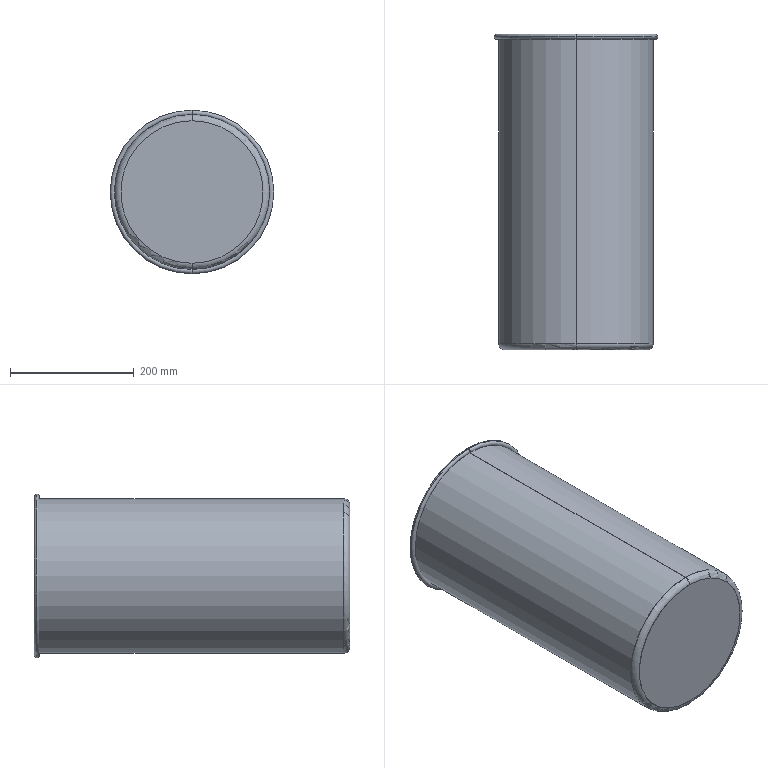Part | SolidWorks | features Extrusion 1, Fillet 1, Revolution 1, Shell 1 | 2 solids | 19 faces | box 264 x 509 x 264 mm | volume 457801 mm3 | torus 12 | cylinder 4 | plane 3 | commonest cylinder face diameters 248 x2 250 x2
STEP:
#1=CARTESIAN_POINT('',(0.,1.,115.));
#2=VERTEX_POINT('',#1);
#3=CARTESIAN_POINT('',(0.,1.,-115.));
#4=VERTEX_POINT('',#3);
#5=CARTESIAN_POINT('',(0.,1.,0.));
#6=DIRECTION('',(0.,-1.,0.));
#7=DIRECTION('',(0.,0.,1.));
#8=AXIS2_PLACEMENT_3D('',#5,#6,#7);
#9=CIRCLE('',#8,115.);
#10=EDGE_CURVE('',#2,#4,#9,.T.);
#11=ORIENTED_EDGE('',*,*,#10,.T.);
#12=CARTESIAN_POINT('',(0.,10.,-124.));
#13=VERTEX_POINT('',#12);
#14=CARTESIAN_POINT('',(0.,10.,-115.));
#15=DIRECTION('',(1.,0.,0.));
#16=DIRECTION('',(0.,0.,-1.));
#17=AXIS2_PLACEMENT_3D('',#14,#15,#16);
#18=CIRCLE('',#17,9.);
#19=EDGE_CURVE('',#4,#13,#18,.T.);
#20=ORIENTED_EDGE('',*,*,#19,.T.);
#21=CARTESIAN_POINT('',(0.,10.,124.));
#22=VERTEX_POINT('',#21);
#23=CARTESIAN_POINT('',(0.,10.,0.));
#24=DIRECTION('',(0.,1.,0.));
#25=DIRECTION('',(0.,0.,-1.));
#26=AXIS2_PLACEMENT_3D('',#23,#24,#25);
#27=CIRCLE('',#26,124.);
#28=EDGE_CURVE('',#13,#22,#27,.T.);
#29=ORIENTED_EDGE('',*,*,#28,.T.);
#30=CARTESIAN_POINT('',(0.,10.,115.));
#31=DIRECTION('',(-1.,0.,0.));
#32=DIRECTION('',(0.,0.,1.));
#33=AXIS2_PLACEMENT_3D('',#30,#31,#32);
#34=CIRCLE('',#33,9.);
#35=EDGE_CURVE('',#2,#22,#34,.T.);
#36=ORIENTED_EDGE('',*,*,#35,.F.);
#37=EDGE_LOOP('',(#11,#20,#29,#36));
#38=FACE_OUTER_BOUND('',#37,.T.);
#39=CARTESIAN_POINT('',(0.,10.,0.));
#40=DIRECTION('',(0.,1.,0.));
#41=DIRECTION('',(0.,0.,1.));
#42=AXIS2_PLACEMENT_3D('',#39,#40,#41);
#43=TOROIDAL_SURFACE('',#42,115.,9.);
#44=ADVANCED_FACE('',(#38),#43,.F.);
#45=CARTESIAN_POINT('',(0.,505.,-124.));
#46=VERTEX_POINT('',#45);
#47=CARTESIAN_POINT('',(0.,505.,124.));
#48=VERTEX_POINT('',#47);
#49=CARTESIAN_POINT('',(0.,505.,0.));
#50=DIRECTION('',(0.,1.,0.));
#51=DIRECTION('',(0.,0.,1.));
#52=AXIS2_PLACEMENT_3D('',#49,#50,#51);
#53=CIRCLE('',#52,124.);
#54=EDGE_CURVE('',#46,#48,#53,.T.);
#55=ORIENTED_EDGE('',*,*,#54,.T.);
#56=CARTESIAN_POINT('',(0.,505.,124.));
#57=DIRECTION('',(0.,-1.,0.));
#58=VECTOR('',#57,1000.);
#59=LINE('',#56,#58);
#60=EDGE_CURVE('',#48,#22,#59,.T.);
#61=ORIENTED_EDGE('',*,*,#60,.T.);
#62=ORIENTED_EDGE('',*,*,#28,.F.);
#63=CARTESIAN_POINT('',(0.,505.,-124.));
#64=DIRECTION('',(0.,-1.,0.));
#65=VECTOR('',#64,1000.);
#66=LINE('',#63,#65);
#67=EDGE_CURVE('',#46,#13,#66,.T.);
#68=ORIENTED_EDGE('',*,*,#67,.F.);
#69=EDGE_LOOP('',(#55,#61,#62,#68));
#70=FACE_OUTER_BOUND('',#69,.T.);
#71=CARTESIAN_POINT('',(0.,505.,0.));
#72=DIRECTION('',(0.,-1.,0.));
#73=DIRECTION('',(0.,0.,-1.));
#74=AXIS2_PLACEMENT_3D('',#71,#72,#73);
#75=CYLINDRICAL_SURFACE('',#74,124.);
#76=ADVANCED_FACE('',(#70),#75,.F.);
#77=CARTESIAN_POINT('',(0.,0.,-115.));
#78=VERTEX_POINT('',#77);
#79=CARTESIAN_POINT('',(0.,0.,115.));
#80=VERTEX_POINT('',#79);
#81=CARTESIAN_POINT('',(0.,0.,0.));
#82=DIRECTION('',(0.,-1.,0.));
#83=DIRECTION('',(0.,0.,1.));
#84=AXIS2_PLACEMENT_3D('',#81,#82,#83);
#85=CIRCLE('',#84,115.);
#86=EDGE_CURVE('',#78,#80,#85,.T.);
#87=ORIENTED_EDGE('',*,*,#86,.F.);
#88=CARTESIAN_POINT('',(0.,10.,-125.));
#89=VERTEX_POINT('',#88);
#90=CARTESIAN_POINT('',(0.,10.,-115.));
#91=DIRECTION('',(1.,0.,0.));
#92=DIRECTION('',(0.,0.,-1.));
#93=AXIS2_PLACEMENT_3D('',#90,#91,#92);
#94=CIRCLE('',#93,10.);
#95=EDGE_CURVE('',#78,#89,#94,.T.);
#96=ORIENTED_EDGE('',*,*,#95,.T.);
#97=CARTESIAN_POINT('',(0.,10.,125.));
#98=VERTEX_POINT('',#97);
#99=CARTESIAN_POINT('',(0.,10.,0.));
#100=DIRECTION('',(0.,1.,0.));
#101=DIRECTION('',(0.,0.,1.));
#102=AXIS2_PLACEMENT_3D('',#99,#100,#101);
#103=CIRCLE('',#102,125.);
#104=EDGE_CURVE('',#98,#89,#103,.T.);
#105=ORIENTED_EDGE('',*,*,#104,.F.);
#106=CARTESIAN_POINT('',(0.,10.,115.));
#107=DIRECTION('',(-1.,0.,0.));
#108=DIRECTION('',(0.,0.,1.));
#109=AXIS2_PLACEMENT_3D('',#106,#107,#108);
#110=CIRCLE('',#109,10.);
#111=EDGE_CURVE('',#80,#98,#110,.T.);
#112=ORIENTED_EDGE('',*,*,#111,.F.);
#113=EDGE_LOOP('',(#87,#96,#105,#112));
#114=FACE_OUTER_BOUND('',#113,.T.);
#115=CARTESIAN_POINT('',(0.,10.,0.));
#116=DIRECTION('',(0.,1.,0.));
#117=DIRECTION('',(0.,0.,1.));
#118=AXIS2_PLACEMENT_3D('',#115,#116,#117);
#119=TOROIDAL_SURFACE('',#118,115.,10.);
#120=ADVANCED_FACE('',(#114),#119,.T.);
#121=CARTESIAN_POINT('',(0.,505.,125.));
#122=VERTEX_POINT('',#121);
#123=CARTESIAN_POINT('',(0.,505.,-125.));
#124=VERTEX_POINT('',#123);
#125=CARTESIAN_POINT('',(0.,505.,0.));
#126=DIRECTION('',(0.,1.,0.));
#127=DIRECTION('',(0.,0.,1.));
#128=AXIS2_PLACEMENT_3D('',#125,#126,#127);
#129=CIRCLE('',#128,125.);
#130=EDGE_CURVE('',#122,#124,#129,.T.);
#131=ORIENTED_EDGE('',*,*,#130,.F.);
#132=CARTESIAN_POINT('',(0.,505.,125.));
#133=DIRECTION('',(0.,-1.,0.));
#134=VECTOR('',#133,1000.);
#135=LINE('',#132,#134);
#136=EDGE_CURVE('',#122,#98,#135,.T.);
#137=ORIENTED_EDGE('',*,*,#136,.T.);
#138=ORIENTED_EDGE('',*,*,#104,.T.);
#139=CARTESIAN_POINT('',(0.,505.,-125.));
#140=DIRECTION('',(0.,-1.,0.));
#141=VECTOR('',#140,1000.);
#142=LINE('',#139,#141);
#143=EDGE_CURVE('',#124,#89,#142,.T.);
#144=ORIENTED_EDGE('',*,*,#143,.F.);
#145=EDGE_LOOP('',(#131,#137,#138,#144));
#146=FACE_OUTER_BOUND('',#145,.T.);
#147=CARTESIAN_POINT('',(0.,505.,0.));
#148=DIRECTION('',(0.,-1.,0.));
#149=DIRECTION('',(0.,0.,-1.));
#150=AXIS2_PLACEMENT_3D('',#147,#148,#149);
#151=CYLINDRICAL_SURFACE('',#150,125.);
#152=ADVANCED_FACE('',(#146),#151,.T.);
#153=ORIENTED_EDGE('',*,*,#136,.F.);
#154=CARTESIAN_POINT('',(0.,505.,0.));
#155=DIRECTION('',(0.,1.,0.));
#156=DIRECTION('',(0.,0.,1.));
#157=AXIS2_PLACEMENT_3D('',#154,#155,#156);
#158=CIRCLE('',#157,125.);
#159=EDGE_CURVE('',#124,#122,#158,.T.);
#160=ORIENTED_EDGE('',*,*,#159,.F.);
#161=ORIENTED_EDGE('',*,*,#143,.T.);
#162=CARTESIAN_POINT('',(0.,10.,0.));
#163=DIRECTION('',(0.,1.,0.));
#164=DIRECTION('',(0.,0.,1.));
#165=AXIS2_PLACEMENT_3D('',#162,#163,#164);
#166=CIRCLE('',#165,125.);
#167=EDGE_CURVE('',#89,#98,#166,.T.);
#168=ORIENTED_EDGE('',*,*,#167,.T.);
#169=EDGE_LOOP('',(#153,#160,#161,#168));
#170=FACE_OUTER_BOUND('',#169,.T.);
#171=CARTESIAN_POINT('',(0.,505.,0.));
#172=DIRECTION('',(0.,-1.,0.));
#173=DIRECTION('',(0.,0.,-1.));
#174=AXIS2_PLACEMENT_3D('',#171,#172,#173);
#175=CYLINDRICAL_SURFACE('',#174,125.);
#176=ADVANCED_FACE('',(#170),#175,.T.);
#177=ORIENTED_EDGE('',*,*,#54,.F.);
#178=CARTESIAN_POINT('',(0.,505.,0.));
#179=DIRECTION('',(0.,1.,0.));
#180=DIRECTION('',(0.,0.,1.));
#181=AXIS2_PLACEMENT_3D('',#178,#179,#180);
#182=CIRCLE('',#181,124.);
#183=EDGE_CURVE('',#48,#46,#182,.T.);
#184=ORIENTED_EDGE('',*,*,#183,.F.);
#185=EDGE_LOOP('',(#177,#184));
#186=FACE_BOUND('',#185,.T.);
#187=ORIENTED_EDGE('',*,*,#159,.T.);
#188=ORIENTED_EDGE('',*,*,#130,.T.);
#189=EDGE_LOOP('',(#187,#188));
#190=FACE_OUTER_BOUND('',#189,.T.);
#191=CARTESIAN_POINT('',(0.,505.,0.));
#192=DIRECTION('',(0.,1.,0.));
#193=DIRECTION('',(0.,0.,1.));
#194=AXIS2_PLACEMENT_3D('',#191,#192,#193);
#195=PLANE('',#194);
#196=ADVANCED_FACE('',(#186,#190),#195,.T.);
#197=CARTESIAN_POINT('',(0.,0.,0.));
#198=DIRECTION('',(0.,-1.,0.));
#199=DIRECTION('',(0.,0.,1.));
#200=AXIS2_PLACEMENT_3D('',#197,#198,#199);
#201=CIRCLE('',#200,115.);
#202=EDGE_CURVE('',#80,#78,#201,.T.);
#203=ORIENTED_EDGE('',*,*,#202,.T.);
#204=ORIENTED_EDGE('',*,*,#86,.T.);
#205=EDGE_LOOP('',(#203,#204));
#206=FACE_OUTER_BOUND('',#205,.T.);
#207=CARTESIAN_POINT('',(0.,0.,0.));
#208=DIRECTION('',(0.,1.,0.));
#209=DIRECTION('',(0.,0.,1.));
#210=AXIS2_PLACEMENT_3D('',#207,#208,#209);
#211=PLANE('',#210);
#212=ADVANCED_FACE('',(#206),#211,.F.);
#213=ORIENTED_EDGE('',*,*,#95,.F.);
#214=ORIENTED_EDGE('',*,*,#202,.F.);
#215=ORIENTED_EDGE('',*,*,#111,.T.);
#216=ORIENTED_EDGE('',*,*,#167,.F.);
#217=EDGE_LOOP('',(#213,#214,#215,#216));
#218=FACE_OUTER_BOUND('',#217,.T.);
#219=CARTESIAN_POINT('',(0.,10.,0.));
#220=DIRECTION('',(0.,1.,0.));
#221=DIRECTION('',(0.,0.,1.));
#222=AXIS2_PLACEMENT_3D('',#219,#220,#221);
#223=TOROIDAL_SURFACE('',#222,115.,10.);
#224=ADVANCED_FACE('',(#218),#223,.T.);
#225=ORIENTED_EDGE('',*,*,#60,.F.);
#226=ORIENTED_EDGE('',*,*,#183,.T.);
#227=ORIENTED_EDGE('',*,*,#67,.T.);
#228=CARTESIAN_POINT('',(0.,10.,0.));
#229=DIRECTION('',(0.,1.,0.));
#230=DIRECTION('',(0.,0.,-1.));
#231=AXIS2_PLACEMENT_3D('',#228,#229,#230);
#232=CIRCLE('',#231,124.);
#233=EDGE_CURVE('',#22,#13,#232,.T.);
#234=ORIENTED_EDGE('',*,*,#233,.F.);
#235=EDGE_LOOP('',(#225,#226,#227,#234));
#236=FACE_OUTER_BOUND('',#235,.T.);
#237=CARTESIAN_POINT('',(0.,505.,0.));
#238=DIRECTION('',(0.,-1.,0.));
#239=DIRECTION('',(0.,0.,-1.));
#240=AXIS2_PLACEMENT_3D('',#237,#238,#239);
#241=CYLINDRICAL_SURFACE('',#240,124.);
#242=ADVANCED_FACE('',(#236),#241,.F.);
#243=ORIENTED_EDGE('',*,*,#10,.F.);
#244=CARTESIAN_POINT('',(0.,1.,0.));
#245=DIRECTION('',(0.,-1.,0.));
#246=DIRECTION('',(0.,0.,1.));
#247=AXIS2_PLACEMENT_3D('',#244,#245,#246);
#248=CIRCLE('',#247,115.);
#249=EDGE_CURVE('',#4,#2,#248,.T.);
#250=ORIENTED_EDGE('',*,*,#249,.F.);
#251=EDGE_LOOP('',(#243,#250));
#252=FACE_OUTER_BOUND('',#251,.T.);
#253=CARTESIAN_POINT('',(0.,1.,0.));
#254=DIRECTION('',(0.,1.,0.));
#255=DIRECTION('',(0.,0.,1.));
#256=AXIS2_PLACEMENT_3D('',#253,#254,#255);
#257=PLANE('',#256);
#258=ADVANCED_FACE('',(#252),#257,.T.);
#259=ORIENTED_EDGE('',*,*,#19,.F.);
#260=ORIENTED_EDGE('',*,*,#249,.T.);
#261=ORIENTED_EDGE('',*,*,#35,.T.);
#262=ORIENTED_EDGE('',*,*,#233,.T.);
#263=EDGE_LOOP('',(#259,#260,#261,#262));
#264=FACE_OUTER_BOUND('',#263,.T.);
#265=CARTESIAN_POINT('',(0.,10.,0.));
#266=DIRECTION('',(0.,1.,0.));
#267=DIRECTION('',(0.,0.,1.));
#268=AXIS2_PLACEMENT_3D('',#265,#266,#267);
#269=TOROIDAL_SURFACE('',#268,115.,9.);
#270=ADVANCED_FACE('',(#264),#269,.F.);
#271=CLOSED_SHELL('',(#44,#76,#120,#152,#176,#196,#212,#224,#242,#258,#270));
#272=MANIFOLD_SOLID_BREP('',#271);
#273=CARTESIAN_POINT('',(0.,505.,132.));
#274=VERTEX_POINT('',#273);
#275=CARTESIAN_POINT('',(0.,505.,124.));
#276=VERTEX_POINT('',#275);
#277=CARTESIAN_POINT('',(0.,505.,128.));
#278=DIRECTION('',(1.,0.,0.));
#279=DIRECTION('',(0.,0.,-1.));
#280=AXIS2_PLACEMENT_3D('',#277,#278,#279);
#281=CIRCLE('',#280,4.);
#282=EDGE_CURVE('',#274,#276,#281,.T.);
#283=ORIENTED_EDGE('',*,*,#282,.F.);
#284=CARTESIAN_POINT('',(0.,505.,-132.));
#285=VERTEX_POINT('',#284);
#286=CARTESIAN_POINT('',(0.,505.,0.));
#287=DIRECTION('',(0.,-1.,0.));
#288=DIRECTION('',(0.,0.,-1.));
#289=AXIS2_PLACEMENT_3D('',#286,#287,#288);
#290=CIRCLE('',#289,132.);
#291=EDGE_CURVE('',#274,#285,#290,.T.);
#292=ORIENTED_EDGE('',*,*,#291,.T.);
#293=CARTESIAN_POINT('',(0.,505.,-124.));
#294=VERTEX_POINT('',#293);
#295=CARTESIAN_POINT('',(0.,505.,-128.));
#296=DIRECTION('',(-1.,0.,0.));
#297=DIRECTION('',(0.,0.,1.));
#298=AXIS2_PLACEMENT_3D('',#295,#296,#297);
#299=CIRCLE('',#298,4.);
#300=EDGE_CURVE('',#285,#294,#299,.T.);
#301=ORIENTED_EDGE('',*,*,#300,.T.);
#302=CARTESIAN_POINT('',(0.,505.,0.));
#303=DIRECTION('',(0.,-1.,0.));
#304=DIRECTION('',(0.,0.,-1.));
#305=AXIS2_PLACEMENT_3D('',#302,#303,#304);
#306=CIRCLE('',#305,124.);
#307=EDGE_CURVE('',#276,#294,#306,.T.);
#308=ORIENTED_EDGE('',*,*,#307,.F.);
#309=EDGE_LOOP('',(#283,#292,#301,#308));
#310=FACE_OUTER_BOUND('',#309,.T.);
#311=CARTESIAN_POINT('',(0.,505.,0.));
#312=DIRECTION('',(0.,-1.,0.));
#313=DIRECTION('',(0.,0.,-1.));
#314=AXIS2_PLACEMENT_3D('',#311,#312,#313);
#315=TOROIDAL_SURFACE('',#314,128.,4.);
#316=ADVANCED_FACE('',(#310),#315,.T.);
#317=ORIENTED_EDGE('',*,*,#300,.F.);
#318=CARTESIAN_POINT('',(0.,505.,0.));
#319=DIRECTION('',(0.,-1.,0.));
#320=DIRECTION('',(0.,0.,-1.));
#321=AXIS2_PLACEMENT_3D('',#318,#319,#320);
#322=CIRCLE('',#321,132.);
#323=EDGE_CURVE('',#285,#274,#322,.T.);
#324=ORIENTED_EDGE('',*,*,#323,.T.);
#325=ORIENTED_EDGE('',*,*,#282,.T.);
#326=CARTESIAN_POINT('',(0.,505.,0.));
#327=DIRECTION('',(0.,-1.,0.));
#328=DIRECTION('',(0.,0.,-1.));
#329=AXIS2_PLACEMENT_3D('',#326,#327,#328);
#330=CIRCLE('',#329,124.);
#331=EDGE_CURVE('',#294,#276,#330,.T.);
#332=ORIENTED_EDGE('',*,*,#331,.F.);
#333=EDGE_LOOP('',(#317,#324,#325,#332));
#334=FACE_OUTER_BOUND('',#333,.T.);
#335=CARTESIAN_POINT('',(0.,505.,0.));
#336=DIRECTION('',(0.,-1.,0.));
#337=DIRECTION('',(0.,0.,-1.));
#338=AXIS2_PLACEMENT_3D('',#335,#336,#337);
#339=TOROIDAL_SURFACE('',#338,128.,4.);
#340=ADVANCED_FACE('',(#334),#339,.T.);
#341=ORIENTED_EDGE('',*,*,#323,.F.);
#342=CARTESIAN_POINT('',(0.,505.,-128.));
#343=DIRECTION('',(-1.,0.,0.));
#344=DIRECTION('',(0.,0.,1.));
#345=AXIS2_PLACEMENT_3D('',#342,#343,#344);
#346=CIRCLE('',#345,4.);
#347=EDGE_CURVE('',#294,#285,#346,.T.);
#348=ORIENTED_EDGE('',*,*,#347,.F.);
#349=ORIENTED_EDGE('',*,*,#331,.T.);
#350=CARTESIAN_POINT('',(0.,505.,128.));
#351=DIRECTION('',(1.,0.,0.));
#352=DIRECTION('',(0.,0.,-1.));
#353=AXIS2_PLACEMENT_3D('',#350,#351,#352);
#354=CIRCLE('',#353,4.);
#355=EDGE_CURVE('',#276,#274,#354,.T.);
#356=ORIENTED_EDGE('',*,*,#355,.T.);
#357=EDGE_LOOP('',(#341,#348,#349,#356));
#358=FACE_OUTER_BOUND('',#357,.T.);
#359=CARTESIAN_POINT('',(0.,505.,0.));
#360=DIRECTION('',(0.,-1.,0.));
#361=DIRECTION('',(0.,0.,-1.));
#362=AXIS2_PLACEMENT_3D('',#359,#360,#361);
#363=TOROIDAL_SURFACE('',#362,128.,4.);
#364=ADVANCED_FACE('',(#358),#363,.T.);
#365=ORIENTED_EDGE('',*,*,#291,.F.);
#366=ORIENTED_EDGE('',*,*,#355,.F.);
#367=ORIENTED_EDGE('',*,*,#307,.T.);
#368=ORIENTED_EDGE('',*,*,#347,.T.);
#369=EDGE_LOOP('',(#365,#366,#367,#368));
#370=FACE_OUTER_BOUND('',#369,.T.);
#371=CARTESIAN_POINT('',(0.,505.,0.));
#372=DIRECTION('',(0.,-1.,0.));
#373=DIRECTION('',(0.,0.,-1.));
#374=AXIS2_PLACEMENT_3D('',#371,#372,#373);
#375=TOROIDAL_SURFACE('',#374,128.,4.);
#376=ADVANCED_FACE('',(#370),#375,.T.);
#377=CLOSED_SHELL('',(#316,#340,#364,#376));
#378=CARTESIAN_POINT('',(0.,505.,-125.));
#379=VERTEX_POINT('',#378);
#380=CARTESIAN_POINT('',(0.,505.,-131.));
#381=VERTEX_POINT('',#380);
#382=CARTESIAN_POINT('',(0.,505.,-128.));
#383=DIRECTION('',(-1.,0.,0.));
#384=DIRECTION('',(0.,0.,1.));
#385=AXIS2_PLACEMENT_3D('',#382,#383,#384);
#386=CIRCLE('',#385,3.);
#387=EDGE_CURVE('',#379,#381,#386,.T.);
#388=ORIENTED_EDGE('',*,*,#387,.T.);
#389=CARTESIAN_POINT('',(0.,505.,131.));
#390=VERTEX_POINT('',#389);
#391=CARTESIAN_POINT('',(0.,505.,0.));
#392=DIRECTION('',(0.,-1.,0.));
#393=DIRECTION('',(0.,0.,-1.));
#394=AXIS2_PLACEMENT_3D('',#391,#392,#393);
#395=CIRCLE('',#394,131.);
#396=EDGE_CURVE('',#381,#390,#395,.T.);
#397=ORIENTED_EDGE('',*,*,#396,.T.);
#398=CARTESIAN_POINT('',(0.,505.,125.));
#399=VERTEX_POINT('',#398);
#400=CARTESIAN_POINT('',(0.,505.,128.));
#401=DIRECTION('',(1.,0.,0.));
#402=DIRECTION('',(0.,0.,-1.));
#403=AXIS2_PLACEMENT_3D('',#400,#401,#402);
#404=CIRCLE('',#403,3.);
#405=EDGE_CURVE('',#399,#390,#404,.T.);
#406=ORIENTED_EDGE('',*,*,#405,.F.);
#407=CARTESIAN_POINT('',(0.,505.,0.));
#408=DIRECTION('',(0.,-1.,0.));
#409=DIRECTION('',(0.,0.,-1.));
#410=AXIS2_PLACEMENT_3D('',#407,#408,#409);
#411=CIRCLE('',#410,125.);
#412=EDGE_CURVE('',#379,#399,#411,.T.);
#413=ORIENTED_EDGE('',*,*,#412,.F.);
#414=EDGE_LOOP('',(#388,#397,#406,#413));
#415=FACE_OUTER_BOUND('',#414,.T.);
#416=CARTESIAN_POINT('',(0.,505.,0.));
#417=DIRECTION('',(0.,-1.,0.));
#418=DIRECTION('',(0.,0.,-1.));
#419=AXIS2_PLACEMENT_3D('',#416,#417,#418);
#420=TOROIDAL_SURFACE('',#419,128.,3.);
#421=ADVANCED_FACE('',(#415),#420,.F.);
#422=ORIENTED_EDGE('',*,*,#405,.T.);
#423=CARTESIAN_POINT('',(0.,505.,0.));
#424=DIRECTION('',(0.,-1.,0.));
#425=DIRECTION('',(0.,0.,-1.));
#426=AXIS2_PLACEMENT_3D('',#423,#424,#425);
#427=CIRCLE('',#426,131.);
#428=EDGE_CURVE('',#390,#381,#427,.T.);
#429=ORIENTED_EDGE('',*,*,#428,.T.);
#430=ORIENTED_EDGE('',*,*,#387,.F.);
#431=CARTESIAN_POINT('',(0.,505.,0.));
#432=DIRECTION('',(0.,-1.,0.));
#433=DIRECTION('',(0.,0.,-1.));
#434=AXIS2_PLACEMENT_3D('',#431,#432,#433);
#435=CIRCLE('',#434,125.);
#436=EDGE_CURVE('',#399,#379,#435,.T.);
#437=ORIENTED_EDGE('',*,*,#436,.F.);
#438=EDGE_LOOP('',(#422,#429,#430,#437));
#439=FACE_OUTER_BOUND('',#438,.T.);
#440=CARTESIAN_POINT('',(0.,505.,0.));
#441=DIRECTION('',(0.,-1.,0.));
#442=DIRECTION('',(0.,0.,-1.));
#443=AXIS2_PLACEMENT_3D('',#440,#441,#442);
#444=TOROIDAL_SURFACE('',#443,128.,3.);
#445=ADVANCED_FACE('',(#439),#444,.F.);
#446=ORIENTED_EDGE('',*,*,#428,.F.);
#447=CARTESIAN_POINT('',(0.,505.,128.));
#448=DIRECTION('',(1.,0.,0.));
#449=DIRECTION('',(0.,0.,-1.));
#450=AXIS2_PLACEMENT_3D('',#447,#448,#449);
#451=CIRCLE('',#450,3.);
#452=EDGE_CURVE('',#390,#399,#451,.T.);
#453=ORIENTED_EDGE('',*,*,#452,.T.);
#454=ORIENTED_EDGE('',*,*,#436,.T.);
#455=CARTESIAN_POINT('',(0.,505.,-128.));
#456=DIRECTION('',(-1.,0.,0.));
#457=DIRECTION('',(0.,0.,1.));
#458=AXIS2_PLACEMENT_3D('',#455,#456,#457);
#459=CIRCLE('',#458,3.);
#460=EDGE_CURVE('',#381,#379,#459,.T.);
#461=ORIENTED_EDGE('',*,*,#460,.F.);
#462=EDGE_LOOP('',(#446,#453,#454,#461));
#463=FACE_OUTER_BOUND('',#462,.T.);
#464=CARTESIAN_POINT('',(0.,505.,0.));
#465=DIRECTION('',(0.,-1.,0.));
#466=DIRECTION('',(0.,0.,-1.));
#467=AXIS2_PLACEMENT_3D('',#464,#465,#466);
#468=TOROIDAL_SURFACE('',#467,128.,3.);
#469=ADVANCED_FACE('',(#463),#468,.F.);
#470=ORIENTED_EDGE('',*,*,#396,.F.);
#471=ORIENTED_EDGE('',*,*,#460,.T.);
#472=ORIENTED_EDGE('',*,*,#412,.T.);
#473=ORIENTED_EDGE('',*,*,#452,.F.);
#474=EDGE_LOOP('',(#470,#471,#472,#473));
#475=FACE_OUTER_BOUND('',#474,.T.);
#476=CARTESIAN_POINT('',(0.,505.,0.));
#477=DIRECTION('',(0.,-1.,0.));
#478=DIRECTION('',(0.,0.,-1.));
#479=AXIS2_PLACEMENT_3D('',#476,#477,#478);
#480=TOROIDAL_SURFACE('',#479,128.,3.);
#481=ADVANCED_FACE('',(#475),#480,.F.);
#482=CLOSED_SHELL('',(#421,#445,#469,#481));
#483=ORIENTED_CLOSED_SHELL('',*,#482,.F.);
#484=BREP_WITH_VOIDS('',#377,(#483));
#485=CARTESIAN_POINT('',(0.,0.,0.));
#486=DIRECTION('',(0.,0.,1.));
#487=DIRECTION('',(1.,0.,0.));
#488=AXIS2_PLACEMENT_3D('',#485,#486,#487);
#489=(LENGTH_UNIT()NAMED_UNIT(*)SI_UNIT(.MILLI.,.METRE.));
#490=UNCERTAINTY_MEASURE_WITH_UNIT(LENGTH_MEASURE(0.00001),#489,'','');
#491=(NAMED_UNIT(*)PLANE_ANGLE_UNIT()SI_UNIT($,.RADIAN.));
#492=(NAMED_UNIT(*)SI_UNIT($,.STERADIAN.)SOLID_ANGLE_UNIT());
#493=(GEOMETRIC_REPRESENTATION_CONTEXT(3)GLOBAL_UNCERTAINTY_ASSIGNED_CONTEXT((#490))GLOBAL_UNIT_ASSIGNED_CONTEXT((#489,#491,#492))REPRESENTATION_CONTEXT('',''));
#494=ADVANCED_BREP_SHAPE_REPRESENTATION('',(#272,#484,#488),#493);